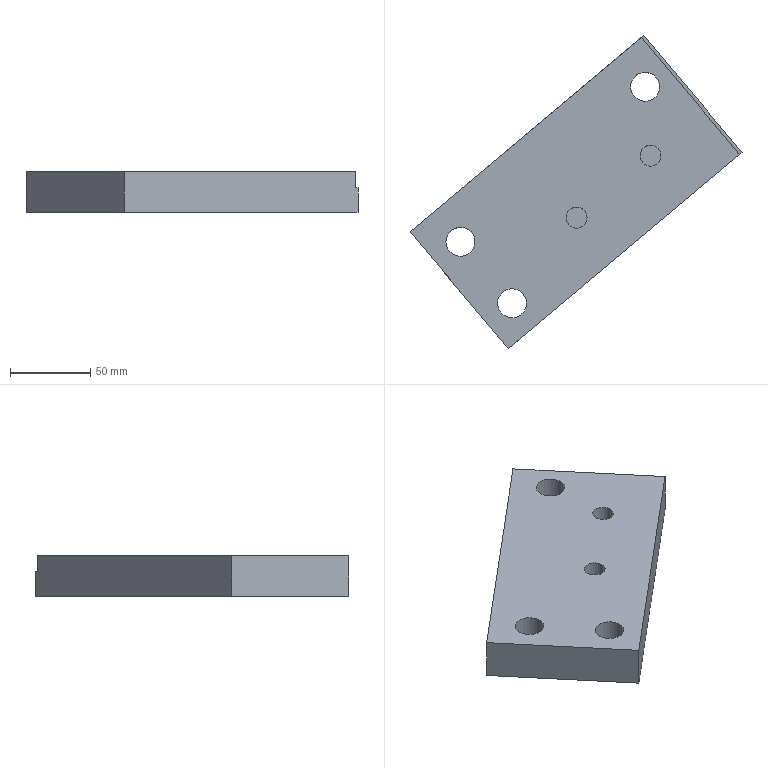Part | NX | features solid 2 | 1 solid | 21 faces | box 206.613 x 194.904 x 25 mm | volume 421657 mm3 | plane 13 | cylinder 8 | commonest cylinder face diameters 18 x3 32 x3 13 x2
STEP:
#1=CARTESIAN_POINT('',(888.592,442.239,75.));
#2=VERTEX_POINT('',#1);
#3=CARTESIAN_POINT('',(886.369,436.131,75.));
#4=DIRECTION('',(0.,0.,1.));
#5=DIRECTION('',(0.342,0.9397,0.));
#6=AXIS2_PLACEMENT_3D('',#3,#4,#5);
#7=CIRCLE('',#6,6.5);
#8=EDGE_CURVE('',#2,#2,#7,.T.);
#9=ORIENTED_EDGE('',*,*,#8,.F.);
#10=EDGE_LOOP('',(#9));
#11=FACE_BOUND('',#10,.T.);
#12=CARTESIAN_POINT('',(771.194,391.051,75.));
#13=VERTEX_POINT('',#12);
#14=CARTESIAN_POINT('',(768.116,382.594,75.));
#15=DIRECTION('',(0.,0.,1.));
#16=DIRECTION('',(0.342,0.9397,0.));
#17=AXIS2_PLACEMENT_3D('',#14,#15,#16);
#18=CIRCLE('',#17,9.);
#19=EDGE_CURVE('',#13,#13,#18,.T.);
#20=ORIENTED_EDGE('',*,*,#19,.F.);
#21=EDGE_LOOP('',(#20));
#22=FACE_BOUND('',#21,.T.);
#23=CARTESIAN_POINT('',(803.333,352.749,75.));
#24=VERTEX_POINT('',#23);
#25=CARTESIAN_POINT('',(800.255,344.292,75.));
#26=DIRECTION('',(0.,0.,1.));
#27=DIRECTION('',(0.342,0.9397,0.));
#28=AXIS2_PLACEMENT_3D('',#25,#26,#27);
#29=CIRCLE('',#28,9.);
#30=EDGE_CURVE('',#24,#24,#29,.T.);
#31=ORIENTED_EDGE('',*,*,#30,.F.);
#32=EDGE_LOOP('',(#31));
#33=FACE_BOUND('',#32,.T.);
#34=CARTESIAN_POINT('',(886.101,487.47,75.));
#35=VERTEX_POINT('',#34);
#36=CARTESIAN_POINT('',(883.022,479.012,75.));
#37=DIRECTION('',(0.,0.,1.));
#38=DIRECTION('',(0.342,0.9397,0.));
#39=AXIS2_PLACEMENT_3D('',#36,#37,#38);
#40=CIRCLE('',#39,9.);
#41=EDGE_CURVE('',#35,#35,#40,.T.);
#42=ORIENTED_EDGE('',*,*,#41,.F.);
#43=EDGE_LOOP('',(#42));
#44=FACE_BOUND('',#43,.T.);
#45=CARTESIAN_POINT('',(880.741,509.734,75.));
#46=VERTEX_POINT('',#45);
#47=CARTESIAN_POINT('',(736.725,388.89,75.));
#48=VERTEX_POINT('',#47);
#49=CARTESIAN_POINT('',(880.741,509.734,75.));
#50=DIRECTION('',(-0.766,-0.6428,0.));
#51=VECTOR('',#50,1000.);
#52=LINE('',#49,#51);
#53=EDGE_CURVE('',#46,#48,#52,.T.);
#54=ORIENTED_EDGE('',*,*,#53,.T.);
#55=CARTESIAN_POINT('',(797.79,316.115,75.));
#56=VERTEX_POINT('',#55);
#57=CARTESIAN_POINT('',(797.79,316.115,75.));
#58=DIRECTION('',(-0.6428,0.766,0.));
#59=VECTOR('',#58,1000.);
#60=LINE('',#57,#59);
#61=EDGE_CURVE('',#56,#48,#60,.T.);
#62=ORIENTED_EDGE('',*,*,#61,.F.);
#63=CARTESIAN_POINT('',(941.806,436.959,75.));
#64=VERTEX_POINT('',#63);
#65=CARTESIAN_POINT('',(941.806,436.959,75.));
#66=DIRECTION('',(-0.766,-0.6428,0.));
#67=VECTOR('',#66,1000.);
#68=LINE('',#65,#67);
#69=EDGE_CURVE('',#64,#56,#68,.T.);
#70=ORIENTED_EDGE('',*,*,#69,.F.);
#71=CARTESIAN_POINT('',(941.806,436.959,75.));
#72=DIRECTION('',(-0.6428,0.766,0.));
#73=VECTOR('',#72,1000.);
#74=LINE('',#71,#73);
#75=EDGE_CURVE('',#64,#46,#74,.T.);
#76=ORIENTED_EDGE('',*,*,#75,.T.);
#77=EDGE_LOOP('',(#54,#62,#70,#76));
#78=FACE_BOUND('',#77,.T.);
#79=CARTESIAN_POINT('',(842.629,403.672,75.));
#80=VERTEX_POINT('',#79);
#81=CARTESIAN_POINT('',(840.406,397.564,75.));
#82=DIRECTION('',(0.,0.,1.));
#83=DIRECTION('',(0.342,0.9397,0.));
#84=AXIS2_PLACEMENT_3D('',#81,#82,#83);
#85=CIRCLE('',#84,6.5);
#86=EDGE_CURVE('',#80,#80,#85,.T.);
#87=ORIENTED_EDGE('',*,*,#86,.F.);
#88=EDGE_LOOP('',(#87));
#89=FACE_BOUND('',#88,.T.);
#90=CARTESIAN_POINT('',(941.806,436.959,75.));
#91=DIRECTION('',(0.,0.,-1.));
#92=DIRECTION('',(0.766,0.6428,0.));
#93=AXIS2_PLACEMENT_3D('',#90,#91,#92);
#94=PLANE('',#93);
#95=ADVANCED_FACE('',(#11,#22,#33,#44,#78,#89),#94,.F.);
#96=CARTESIAN_POINT('',(888.495,494.047,50.));
#97=VERTEX_POINT('',#96);
#98=CARTESIAN_POINT('',(883.022,479.012,50.));
#99=DIRECTION('',(0.,0.,1.));
#100=DIRECTION('',(0.342,0.9397,0.));
#101=AXIS2_PLACEMENT_3D('',#98,#99,#100);
#102=CIRCLE('',#101,16.);
#103=EDGE_CURVE('',#97,#97,#102,.T.);
#104=ORIENTED_EDGE('',*,*,#103,.T.);
#105=EDGE_LOOP('',(#104));
#106=FACE_BOUND('',#105,.T.);
#107=CARTESIAN_POINT('',(773.588,397.629,50.));
#108=VERTEX_POINT('',#107);
#109=CARTESIAN_POINT('',(768.116,382.594,50.));
#110=DIRECTION('',(0.,0.,1.));
#111=DIRECTION('',(0.342,0.9397,0.));
#112=AXIS2_PLACEMENT_3D('',#109,#110,#111);
#113=CIRCLE('',#112,16.);
#114=EDGE_CURVE('',#108,#108,#113,.T.);
#115=ORIENTED_EDGE('',*,*,#114,.T.);
#116=EDGE_LOOP('',(#115));
#117=FACE_BOUND('',#116,.T.);
#118=CARTESIAN_POINT('',(805.727,359.327,50.));
#119=VERTEX_POINT('',#118);
#120=CARTESIAN_POINT('',(800.255,344.292,50.));
#121=DIRECTION('',(0.,0.,1.));
#122=DIRECTION('',(0.342,0.9397,0.));
#123=AXIS2_PLACEMENT_3D('',#120,#121,#122);
#124=CIRCLE('',#123,16.);
#125=EDGE_CURVE('',#119,#119,#124,.T.);
#126=ORIENTED_EDGE('',*,*,#125,.T.);
#127=EDGE_LOOP('',(#126));
#128=FACE_BOUND('',#127,.T.);
#129=CARTESIAN_POINT('',(736.725,388.89,50.));
#130=VERTEX_POINT('',#129);
#131=CARTESIAN_POINT('',(882.274,511.019,50.));
#132=VERTEX_POINT('',#131);
#133=CARTESIAN_POINT('',(736.725,388.89,50.));
#134=DIRECTION('',(0.766,0.6428,0.));
#135=VECTOR('',#134,1000.);
#136=LINE('',#133,#135);
#137=EDGE_CURVE('',#130,#132,#136,.T.);
#138=ORIENTED_EDGE('',*,*,#137,.T.);
#139=CARTESIAN_POINT('',(943.338,438.245,50.));
#140=VERTEX_POINT('',#139);
#141=CARTESIAN_POINT('',(943.338,438.245,50.));
#142=DIRECTION('',(-0.6428,0.766,0.));
#143=VECTOR('',#142,1000.);
#144=LINE('',#141,#143);
#145=EDGE_CURVE('',#140,#132,#144,.T.);
#146=ORIENTED_EDGE('',*,*,#145,.F.);
#147=CARTESIAN_POINT('',(797.79,316.115,50.));
#148=VERTEX_POINT('',#147);
#149=CARTESIAN_POINT('',(797.79,316.115,50.));
#150=DIRECTION('',(0.766,0.6428,0.));
#151=VECTOR('',#150,1000.);
#152=LINE('',#149,#151);
#153=EDGE_CURVE('',#148,#140,#152,.T.);
#154=ORIENTED_EDGE('',*,*,#153,.F.);
#155=CARTESIAN_POINT('',(797.79,316.115,50.));
#156=DIRECTION('',(-0.6428,0.766,0.));
#157=VECTOR('',#156,1000.);
#158=LINE('',#155,#157);
#159=EDGE_CURVE('',#148,#130,#158,.T.);
#160=ORIENTED_EDGE('',*,*,#159,.T.);
#161=EDGE_LOOP('',(#138,#146,#154,#160));
#162=FACE_BOUND('',#161,.T.);
#163=CARTESIAN_POINT('',(797.79,316.115,50.));
#164=DIRECTION('',(0.,0.,1.));
#165=DIRECTION('',(-0.766,-0.6428,0.));
#166=AXIS2_PLACEMENT_3D('',#163,#164,#165);
#167=PLANE('',#166);
#168=ADVANCED_FACE('',(#106,#117,#128,#162),#167,.F.);
#169=CARTESIAN_POINT('',(882.274,511.019,65.));
#170=VERTEX_POINT('',#169);
#171=CARTESIAN_POINT('',(882.274,511.019,50.));
#172=DIRECTION('',(0.,0.,1.));
#173=VECTOR('',#172,1000.);
#174=LINE('',#171,#173);
#175=EDGE_CURVE('',#132,#170,#174,.T.);
#176=ORIENTED_EDGE('',*,*,#175,.T.);
#177=CARTESIAN_POINT('',(943.338,438.245,65.));
#178=VERTEX_POINT('',#177);
#179=CARTESIAN_POINT('',(943.338,438.245,65.));
#180=DIRECTION('',(-0.6428,0.766,0.));
#181=VECTOR('',#180,1000.);
#182=LINE('',#179,#181);
#183=EDGE_CURVE('',#178,#170,#182,.T.);
#184=ORIENTED_EDGE('',*,*,#183,.F.);
#185=CARTESIAN_POINT('',(943.338,438.245,50.));
#186=DIRECTION('',(0.,0.,1.));
#187=VECTOR('',#186,1000.);
#188=LINE('',#185,#187);
#189=EDGE_CURVE('',#140,#178,#188,.T.);
#190=ORIENTED_EDGE('',*,*,#189,.F.);
#191=ORIENTED_EDGE('',*,*,#145,.T.);
#192=EDGE_LOOP('',(#176,#184,#190,#191));
#193=FACE_BOUND('',#192,.T.);
#194=CARTESIAN_POINT('',(943.338,438.245,50.));
#195=DIRECTION('',(-0.766,-0.6428,0.));
#196=DIRECTION('',(0.,0.,-1.));
#197=AXIS2_PLACEMENT_3D('',#194,#195,#196);
#198=PLANE('',#197);
#199=ADVANCED_FACE('',(#193),#198,.F.);
#200=CARTESIAN_POINT('',(880.741,509.734,65.));
#201=VERTEX_POINT('',#200);
#202=CARTESIAN_POINT('',(882.274,511.019,65.));
#203=DIRECTION('',(-0.766,-0.6428,0.));
#204=VECTOR('',#203,1000.);
#205=LINE('',#202,#204);
#206=EDGE_CURVE('',#170,#201,#205,.T.);
#207=ORIENTED_EDGE('',*,*,#206,.T.);
#208=CARTESIAN_POINT('',(941.806,436.959,65.));
#209=VERTEX_POINT('',#208);
#210=CARTESIAN_POINT('',(941.806,436.959,65.));
#211=DIRECTION('',(-0.6428,0.766,0.));
#212=VECTOR('',#211,1000.);
#213=LINE('',#210,#212);
#214=EDGE_CURVE('',#209,#201,#213,.T.);
#215=ORIENTED_EDGE('',*,*,#214,.F.);
#216=CARTESIAN_POINT('',(943.338,438.245,65.));
#217=DIRECTION('',(-0.766,-0.6428,0.));
#218=VECTOR('',#217,1000.);
#219=LINE('',#216,#218);
#220=EDGE_CURVE('',#178,#209,#219,.T.);
#221=ORIENTED_EDGE('',*,*,#220,.F.);
#222=ORIENTED_EDGE('',*,*,#183,.T.);
#223=EDGE_LOOP('',(#207,#215,#221,#222));
#224=FACE_BOUND('',#223,.T.);
#225=CARTESIAN_POINT('',(943.338,438.245,65.));
#226=DIRECTION('',(0.,0.,-1.));
#227=DIRECTION('',(0.766,0.6428,0.));
#228=AXIS2_PLACEMENT_3D('',#225,#226,#227);
#229=PLANE('',#228);
#230=ADVANCED_FACE('',(#224),#229,.F.);
#231=CARTESIAN_POINT('',(880.741,509.734,65.));
#232=DIRECTION('',(0.,0.,1.));
#233=VECTOR('',#232,1000.);
#234=LINE('',#231,#233);
#235=EDGE_CURVE('',#201,#46,#234,.T.);
#236=ORIENTED_EDGE('',*,*,#235,.T.);
#237=ORIENTED_EDGE('',*,*,#75,.F.);
#238=CARTESIAN_POINT('',(941.806,436.959,65.));
#239=DIRECTION('',(0.,0.,1.));
#240=VECTOR('',#239,1000.);
#241=LINE('',#238,#240);
#242=EDGE_CURVE('',#209,#64,#241,.T.);
#243=ORIENTED_EDGE('',*,*,#242,.F.);
#244=ORIENTED_EDGE('',*,*,#214,.T.);
#245=EDGE_LOOP('',(#236,#237,#243,#244));
#246=FACE_BOUND('',#245,.T.);
#247=CARTESIAN_POINT('',(941.806,436.959,65.));
#248=DIRECTION('',(-0.766,-0.6428,0.));
#249=DIRECTION('',(0.,0.,-1.));
#250=AXIS2_PLACEMENT_3D('',#247,#248,#249);
#251=PLANE('',#250);
#252=ADVANCED_FACE('',(#246),#251,.F.);
#253=CARTESIAN_POINT('',(736.725,388.89,75.));
#254=DIRECTION('',(0.,0.,-1.));
#255=VECTOR('',#254,1000.);
#256=LINE('',#253,#255);
#257=EDGE_CURVE('',#48,#130,#256,.T.);
#258=ORIENTED_EDGE('',*,*,#257,.T.);
#259=ORIENTED_EDGE('',*,*,#159,.F.);
#260=CARTESIAN_POINT('',(797.79,316.115,75.));
#261=DIRECTION('',(0.,0.,-1.));
#262=VECTOR('',#261,1000.);
#263=LINE('',#260,#262);
#264=EDGE_CURVE('',#56,#148,#263,.T.);
#265=ORIENTED_EDGE('',*,*,#264,.F.);
#266=ORIENTED_EDGE('',*,*,#61,.T.);
#267=EDGE_LOOP('',(#258,#259,#265,#266));
#268=FACE_BOUND('',#267,.T.);
#269=CARTESIAN_POINT('',(797.79,316.115,75.));
#270=DIRECTION('',(0.766,0.6428,0.));
#271=DIRECTION('',(0.,0.,1.));
#272=AXIS2_PLACEMENT_3D('',#269,#270,#271);
#273=PLANE('',#272);
#274=ADVANCED_FACE('',(#268),#273,.F.);
#275=ORIENTED_EDGE('',*,*,#153,.T.);
#276=ORIENTED_EDGE('',*,*,#189,.T.);
#277=ORIENTED_EDGE('',*,*,#220,.T.);
#278=ORIENTED_EDGE('',*,*,#242,.T.);
#279=ORIENTED_EDGE('',*,*,#69,.T.);
#280=ORIENTED_EDGE('',*,*,#264,.T.);
#281=EDGE_LOOP('',(#275,#276,#277,#278,#279,#280));
#282=FACE_BOUND('',#281,.T.);
#283=CARTESIAN_POINT('',(894.312,397.107,63.333));
#284=DIRECTION('',(0.6428,-0.766,0.));
#285=DIRECTION('',(0.,0.,1.));
#286=AXIS2_PLACEMENT_3D('',#283,#284,#285);
#287=PLANE('',#286);
#288=ADVANCED_FACE('',(#282),#287,.T.);
#289=ORIENTED_EDGE('',*,*,#137,.F.);
#290=ORIENTED_EDGE('',*,*,#257,.F.);
#291=ORIENTED_EDGE('',*,*,#53,.F.);
#292=ORIENTED_EDGE('',*,*,#235,.F.);
#293=ORIENTED_EDGE('',*,*,#206,.F.);
#294=ORIENTED_EDGE('',*,*,#175,.F.);
#295=EDGE_LOOP('',(#289,#290,#291,#292,#293,#294));
#296=FACE_BOUND('',#295,.T.);
#297=CARTESIAN_POINT('',(833.247,469.881,63.333));
#298=DIRECTION('',(0.6428,-0.766,0.));
#299=DIRECTION('',(0.,0.,1.));
#300=AXIS2_PLACEMENT_3D('',#297,#298,#299);
#301=PLANE('',#300);
#302=ADVANCED_FACE('',(#296),#301,.F.);
#303=ORIENTED_EDGE('',*,*,#125,.F.);
#304=EDGE_LOOP('',(#303));
#305=FACE_BOUND('',#304,.T.);
#306=CARTESIAN_POINT('',(805.727,359.327,52.));
#307=VERTEX_POINT('',#306);
#308=CARTESIAN_POINT('',(800.255,344.292,52.));
#309=DIRECTION('',(0.,0.,1.));
#310=DIRECTION('',(0.342,0.9397,0.));
#311=AXIS2_PLACEMENT_3D('',#308,#309,#310);
#312=CIRCLE('',#311,16.);
#313=EDGE_CURVE('',#307,#307,#312,.T.);
#314=ORIENTED_EDGE('',*,*,#313,.T.);
#315=EDGE_LOOP('',(#314));
#316=FACE_BOUND('',#315,.T.);
#317=CARTESIAN_POINT('',(800.255,344.292,50.));
#318=DIRECTION('',(0.,0.,1.));
#319=DIRECTION('',(0.342,0.9397,0.));
#320=AXIS2_PLACEMENT_3D('',#317,#318,#319);
#321=CYLINDRICAL_SURFACE('',#320,16.);
#322=ADVANCED_FACE('',(#305,#316),#321,.F.);
#323=CARTESIAN_POINT('',(803.333,352.749,52.));
#324=VERTEX_POINT('',#323);
#325=CARTESIAN_POINT('',(800.255,344.292,52.));
#326=DIRECTION('',(0.,0.,1.));
#327=DIRECTION('',(0.342,0.9397,0.));
#328=AXIS2_PLACEMENT_3D('',#325,#326,#327);
#329=CIRCLE('',#328,9.);
#330=EDGE_CURVE('',#324,#324,#329,.T.);
#331=ORIENTED_EDGE('',*,*,#330,.T.);
#332=EDGE_LOOP('',(#331));
#333=FACE_BOUND('',#332,.T.);
#334=ORIENTED_EDGE('',*,*,#313,.F.);
#335=EDGE_LOOP('',(#334));
#336=FACE_BOUND('',#335,.T.);
#337=CARTESIAN_POINT('',(800.255,344.292,52.));
#338=DIRECTION('',(0.,0.,1.));
#339=DIRECTION('',(0.342,0.9397,0.));
#340=AXIS2_PLACEMENT_3D('',#337,#338,#339);
#341=PLANE('',#340);
#342=ADVANCED_FACE('',(#333,#336),#341,.F.);
#343=ORIENTED_EDGE('',*,*,#114,.F.);
#344=EDGE_LOOP('',(#343));
#345=FACE_BOUND('',#344,.T.);
#346=CARTESIAN_POINT('',(773.588,397.629,52.));
#347=VERTEX_POINT('',#346);
#348=CARTESIAN_POINT('',(768.116,382.594,52.));
#349=DIRECTION('',(0.,0.,1.));
#350=DIRECTION('',(0.342,0.9397,0.));
#351=AXIS2_PLACEMENT_3D('',#348,#349,#350);
#352=CIRCLE('',#351,16.);
#353=EDGE_CURVE('',#347,#347,#352,.T.);
#354=ORIENTED_EDGE('',*,*,#353,.T.);
#355=EDGE_LOOP('',(#354));
#356=FACE_BOUND('',#355,.T.);
#357=CARTESIAN_POINT('',(768.116,382.594,50.));
#358=DIRECTION('',(0.,0.,1.));
#359=DIRECTION('',(0.342,0.9397,0.));
#360=AXIS2_PLACEMENT_3D('',#357,#358,#359);
#361=CYLINDRICAL_SURFACE('',#360,16.);
#362=ADVANCED_FACE('',(#345,#356),#361,.F.);
#363=CARTESIAN_POINT('',(771.194,391.051,52.));
#364=VERTEX_POINT('',#363);
#365=CARTESIAN_POINT('',(768.116,382.594,52.));
#366=DIRECTION('',(0.,0.,1.));
#367=DIRECTION('',(0.342,0.9397,0.));
#368=AXIS2_PLACEMENT_3D('',#365,#366,#367);
#369=CIRCLE('',#368,9.);
#370=EDGE_CURVE('',#364,#364,#369,.T.);
#371=ORIENTED_EDGE('',*,*,#370,.T.);
#372=EDGE_LOOP('',(#371));
#373=FACE_BOUND('',#372,.T.);
#374=ORIENTED_EDGE('',*,*,#353,.F.);
#375=EDGE_LOOP('',(#374));
#376=FACE_BOUND('',#375,.T.);
#377=CARTESIAN_POINT('',(768.116,382.594,52.));
#378=DIRECTION('',(0.,0.,1.));
#379=DIRECTION('',(0.342,0.9397,0.));
#380=AXIS2_PLACEMENT_3D('',#377,#378,#379);
#381=PLANE('',#380);
#382=ADVANCED_FACE('',(#373,#376),#381,.F.);
#383=ORIENTED_EDGE('',*,*,#103,.F.);
#384=EDGE_LOOP('',(#383));
#385=FACE_BOUND('',#384,.T.);
#386=CARTESIAN_POINT('',(888.495,494.047,52.));
#387=VERTEX_POINT('',#386);
#388=CARTESIAN_POINT('',(883.022,479.012,52.));
#389=DIRECTION('',(0.,0.,1.));
#390=DIRECTION('',(0.342,0.9397,0.));
#391=AXIS2_PLACEMENT_3D('',#388,#389,#390);
#392=CIRCLE('',#391,16.);
#393=EDGE_CURVE('',#387,#387,#392,.T.);
#394=ORIENTED_EDGE('',*,*,#393,.T.);
#395=EDGE_LOOP('',(#394));
#396=FACE_BOUND('',#395,.T.);
#397=CARTESIAN_POINT('',(883.022,479.012,50.));
#398=DIRECTION('',(0.,0.,1.));
#399=DIRECTION('',(0.342,0.9397,0.));
#400=AXIS2_PLACEMENT_3D('',#397,#398,#399);
#401=CYLINDRICAL_SURFACE('',#400,16.);
#402=ADVANCED_FACE('',(#385,#396),#401,.F.);
#403=CARTESIAN_POINT('',(886.101,487.47,52.));
#404=VERTEX_POINT('',#403);
#405=CARTESIAN_POINT('',(883.022,479.012,52.));
#406=DIRECTION('',(0.,0.,1.));
#407=DIRECTION('',(0.342,0.9397,0.));
#408=AXIS2_PLACEMENT_3D('',#405,#406,#407);
#409=CIRCLE('',#408,9.);
#410=EDGE_CURVE('',#404,#404,#409,.T.);
#411=ORIENTED_EDGE('',*,*,#410,.T.);
#412=EDGE_LOOP('',(#411));
#413=FACE_BOUND('',#412,.T.);
#414=ORIENTED_EDGE('',*,*,#393,.F.);
#415=EDGE_LOOP('',(#414));
#416=FACE_BOUND('',#415,.T.);
#417=CARTESIAN_POINT('',(883.022,479.012,52.));
#418=DIRECTION('',(0.,0.,1.));
#419=DIRECTION('',(0.342,0.9397,0.));
#420=AXIS2_PLACEMENT_3D('',#417,#418,#419);
#421=PLANE('',#420);
#422=ADVANCED_FACE('',(#413,#416),#421,.F.);
#423=ORIENTED_EDGE('',*,*,#410,.F.);
#424=EDGE_LOOP('',(#423));
#425=FACE_BOUND('',#424,.T.);
#426=ORIENTED_EDGE('',*,*,#41,.T.);
#427=EDGE_LOOP('',(#426));
#428=FACE_BOUND('',#427,.T.);
#429=CARTESIAN_POINT('',(883.022,479.012,52.));
#430=DIRECTION('',(0.,0.,1.));
#431=DIRECTION('',(0.342,0.9397,0.));
#432=AXIS2_PLACEMENT_3D('',#429,#430,#431);
#433=CYLINDRICAL_SURFACE('',#432,9.);
#434=ADVANCED_FACE('',(#425,#428),#433,.F.);
#435=ORIENTED_EDGE('',*,*,#330,.F.);
#436=EDGE_LOOP('',(#435));
#437=FACE_BOUND('',#436,.T.);
#438=ORIENTED_EDGE('',*,*,#30,.T.);
#439=EDGE_LOOP('',(#438));
#440=FACE_BOUND('',#439,.T.);
#441=CARTESIAN_POINT('',(800.255,344.292,52.));
#442=DIRECTION('',(0.,0.,1.));
#443=DIRECTION('',(0.342,0.9397,0.));
#444=AXIS2_PLACEMENT_3D('',#441,#442,#443);
#445=CYLINDRICAL_SURFACE('',#444,9.);
#446=ADVANCED_FACE('',(#437,#440),#445,.F.);
#447=ORIENTED_EDGE('',*,*,#370,.F.);
#448=EDGE_LOOP('',(#447));
#449=FACE_BOUND('',#448,.T.);
#450=ORIENTED_EDGE('',*,*,#19,.T.);
#451=EDGE_LOOP('',(#450));
#452=FACE_BOUND('',#451,.T.);
#453=CARTESIAN_POINT('',(768.116,382.594,52.));
#454=DIRECTION('',(0.,0.,1.));
#455=DIRECTION('',(0.342,0.9397,0.));
#456=AXIS2_PLACEMENT_3D('',#453,#454,#455);
#457=CYLINDRICAL_SURFACE('',#456,9.);
#458=ADVANCED_FACE('',(#449,#452),#457,.F.);
#459=ORIENTED_EDGE('',*,*,#8,.T.);
#460=EDGE_LOOP('',(#459));
#461=FACE_BOUND('',#460,.T.);
#462=CARTESIAN_POINT('',(888.592,442.239,55.));
#463=VERTEX_POINT('',#462);
#464=CARTESIAN_POINT('',(886.369,436.131,55.));
#465=DIRECTION('',(0.,0.,1.));
#466=DIRECTION('',(0.342,0.9397,0.));
#467=AXIS2_PLACEMENT_3D('',#464,#465,#466);
#468=CIRCLE('',#467,6.5);
#469=EDGE_CURVE('',#463,#463,#468,.T.);
#470=ORIENTED_EDGE('',*,*,#469,.F.);
#471=EDGE_LOOP('',(#470));
#472=FACE_BOUND('',#471,.T.);
#473=CARTESIAN_POINT('',(886.369,436.131,75.));
#474=DIRECTION('',(0.,0.,-1.));
#475=DIRECTION('',(0.9962,-0.08716,0.));
#476=AXIS2_PLACEMENT_3D('',#473,#474,#475);
#477=CYLINDRICAL_SURFACE('',#476,6.5);
#478=ADVANCED_FACE('',(#461,#472),#477,.F.);
#479=ORIENTED_EDGE('',*,*,#469,.T.);
#480=EDGE_LOOP('',(#479));
#481=FACE_BOUND('',#480,.T.);
#482=CARTESIAN_POINT('',(886.369,436.131,55.));
#483=DIRECTION('',(0.,0.,1.));
#484=DIRECTION('',(-0.9962,0.08716,0.));
#485=AXIS2_PLACEMENT_3D('',#482,#483,#484);
#486=PLANE('',#485);
#487=ADVANCED_FACE('',(#481),#486,.T.);
#488=ORIENTED_EDGE('',*,*,#86,.T.);
#489=EDGE_LOOP('',(#488));
#490=FACE_BOUND('',#489,.T.);
#491=CARTESIAN_POINT('',(842.629,403.672,55.));
#492=VERTEX_POINT('',#491);
#493=CARTESIAN_POINT('',(840.406,397.564,55.));
#494=DIRECTION('',(0.,0.,1.));
#495=DIRECTION('',(0.342,0.9397,0.));
#496=AXIS2_PLACEMENT_3D('',#493,#494,#495);
#497=CIRCLE('',#496,6.5);
#498=EDGE_CURVE('',#492,#492,#497,.T.);
#499=ORIENTED_EDGE('',*,*,#498,.F.);
#500=EDGE_LOOP('',(#499));
#501=FACE_BOUND('',#500,.T.);
#502=CARTESIAN_POINT('',(840.406,397.564,75.));
#503=DIRECTION('',(0.,0.,-1.));
#504=DIRECTION('',(0.9962,-0.08716,0.));
#505=AXIS2_PLACEMENT_3D('',#502,#503,#504);
#506=CYLINDRICAL_SURFACE('',#505,6.5);
#507=ADVANCED_FACE('',(#490,#501),#506,.F.);
#508=ORIENTED_EDGE('',*,*,#498,.T.);
#509=EDGE_LOOP('',(#508));
#510=FACE_BOUND('',#509,.T.);
#511=CARTESIAN_POINT('',(840.406,397.564,55.));
#512=DIRECTION('',(0.,0.,1.));
#513=DIRECTION('',(-0.9962,0.08716,0.));
#514=AXIS2_PLACEMENT_3D('',#511,#512,#513);
#515=PLANE('',#514);
#516=ADVANCED_FACE('',(#510),#515,.T.);
#517=CLOSED_SHELL('',(#95,#168,#199,#230,#252,#274,#288,#302,#322,#342,#362,#382,#402,#422,#434,#446,#458,#478,#487,#507,#516));
#518=MANIFOLD_SOLID_BREP('',#517);
#519=(LENGTH_UNIT()NAMED_UNIT(*)SI_UNIT(.MILLI.,.METRE.));
#520=UNCERTAINTY_MEASURE_WITH_UNIT(LENGTH_MEASURE(0.00001),#519,'','');
#521=(NAMED_UNIT(*)PLANE_ANGLE_UNIT()SI_UNIT($,.RADIAN.));
#522=(NAMED_UNIT(*)SI_UNIT($,.STERADIAN.)SOLID_ANGLE_UNIT());
#523=(GEOMETRIC_REPRESENTATION_CONTEXT(3)GLOBAL_UNCERTAINTY_ASSIGNED_CONTEXT((#520))GLOBAL_UNIT_ASSIGNED_CONTEXT((#519,#521,#522))REPRESENTATION_CONTEXT('',''));
#524=ADVANCED_BREP_SHAPE_REPRESENTATION('',(#518),#523);